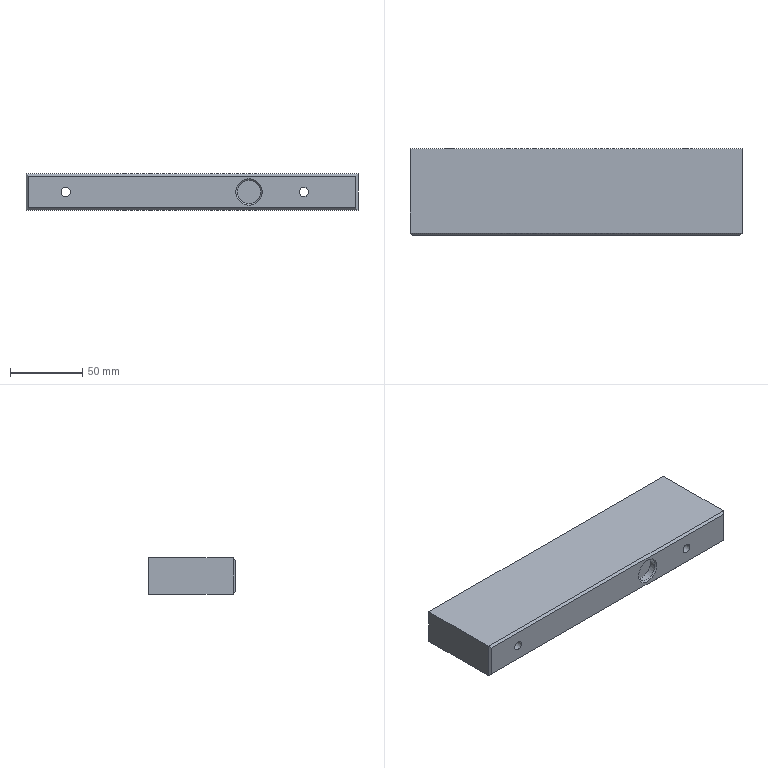Part | NX | 1 solid | 15 faces | box 230 x 60 x 25 mm | volume 339289 mm3 | plane 11 | cylinder 3 | cone 1 | commonest cylinder face diameters 6.5 x2 16.2 x1
STEP:
#1=CARTESIAN_POINT('',(0.,1.5,25.));
#2=VERTEX_POINT('',#1);
#3=CARTESIAN_POINT('',(0.,60.,25.));
#4=VERTEX_POINT('',#3);
#5=CARTESIAN_POINT('',(0.,30.,25.));
#6=DIRECTION('',(0.,1.,0.));
#7=VECTOR('',#6,1000.);
#8=LINE('',#5,#7);
#9=EDGE_CURVE('',#2,#4,#8,.T.);
#10=ORIENTED_EDGE('',*,*,#9,.F.);
#11=CARTESIAN_POINT('',(230.,1.5,25.));
#12=VERTEX_POINT('',#11);
#13=CARTESIAN_POINT('',(115.,1.5,25.));
#14=DIRECTION('',(1.,0.,0.));
#15=VECTOR('',#14,1000.);
#16=LINE('',#13,#15);
#17=EDGE_CURVE('',#2,#12,#16,.T.);
#18=ORIENTED_EDGE('',*,*,#17,.T.);
#19=CARTESIAN_POINT('',(230.,60.,25.));
#20=VERTEX_POINT('',#19);
#21=CARTESIAN_POINT('',(230.,30.,25.));
#22=DIRECTION('',(0.,-1.,0.));
#23=VECTOR('',#22,1000.);
#24=LINE('',#21,#23);
#25=EDGE_CURVE('',#20,#12,#24,.T.);
#26=ORIENTED_EDGE('',*,*,#25,.F.);
#27=CARTESIAN_POINT('',(115.,60.,25.));
#28=DIRECTION('',(1.,0.,0.));
#29=VECTOR('',#28,1000.);
#30=LINE('',#27,#29);
#31=EDGE_CURVE('',#4,#20,#30,.T.);
#32=ORIENTED_EDGE('',*,*,#31,.F.);
#33=EDGE_LOOP('',(#10,#18,#26,#32));
#34=FACE_BOUND('',#33,.T.);
#35=CARTESIAN_POINT('',(115.,30.,25.));
#36=DIRECTION('',(0.,0.,1.));
#37=DIRECTION('',(1.,0.,0.));
#38=AXIS2_PLACEMENT_3D('',#35,#36,#37);
#39=PLANE('',#38);
#40=ADVANCED_FACE('',(#34),#39,.T.);
#41=CARTESIAN_POINT('',(228.5,0.,1.5));
#42=VERTEX_POINT('',#41);
#43=CARTESIAN_POINT('',(228.5,0.,23.5));
#44=VERTEX_POINT('',#43);
#45=CARTESIAN_POINT('',(228.5,0.,0.));
#46=DIRECTION('',(0.,0.,1.));
#47=VECTOR('',#46,1000.);
#48=LINE('',#45,#47);
#49=EDGE_CURVE('',#42,#44,#48,.T.);
#50=ORIENTED_EDGE('',*,*,#49,.T.);
#51=CARTESIAN_POINT('',(1.5,0.,23.5));
#52=VERTEX_POINT('',#51);
#53=CARTESIAN_POINT('',(115.,0.,23.5));
#54=DIRECTION('',(-1.,0.,0.));
#55=VECTOR('',#54,1000.);
#56=LINE('',#53,#55);
#57=EDGE_CURVE('',#44,#52,#56,.T.);
#58=ORIENTED_EDGE('',*,*,#57,.T.);
#59=CARTESIAN_POINT('',(1.5,0.,1.5));
#60=VERTEX_POINT('',#59);
#61=CARTESIAN_POINT('',(1.5,0.,0.));
#62=DIRECTION('',(0.,0.,-1.));
#63=VECTOR('',#62,1000.);
#64=LINE('',#61,#63);
#65=EDGE_CURVE('',#52,#60,#64,.T.);
#66=ORIENTED_EDGE('',*,*,#65,.T.);
#67=CARTESIAN_POINT('',(115.,0.,1.5));
#68=DIRECTION('',(1.,0.,0.));
#69=VECTOR('',#68,1000.);
#70=LINE('',#67,#69);
#71=EDGE_CURVE('',#60,#42,#70,.T.);
#72=ORIENTED_EDGE('',*,*,#71,.T.);
#73=EDGE_LOOP('',(#50,#58,#66,#72));
#74=FACE_BOUND('',#73,.T.);
#75=CARTESIAN_POINT('',(154.5,0.,3.4));
#76=VERTEX_POINT('',#75);
#77=CARTESIAN_POINT('',(154.5,0.,12.5));
#78=DIRECTION('',(0.,-1.,0.));
#79=DIRECTION('',(0.,0.,-1.));
#80=AXIS2_PLACEMENT_3D('',#77,#78,#79);
#81=CIRCLE('',#80,9.1);
#82=EDGE_CURVE('',#76,#76,#81,.F.);
#83=ORIENTED_EDGE('',*,*,#82,.T.);
#84=EDGE_LOOP('',(#83));
#85=FACE_BOUND('',#84,.T.);
#86=CARTESIAN_POINT('',(192.5,0.,15.75));
#87=VERTEX_POINT('',#86);
#88=CARTESIAN_POINT('',(192.5,0.,12.5));
#89=DIRECTION('',(0.,1.,0.));
#90=DIRECTION('',(0.,0.,1.));
#91=AXIS2_PLACEMENT_3D('',#88,#89,#90);
#92=CIRCLE('',#91,3.25);
#93=EDGE_CURVE('',#87,#87,#92,.T.);
#94=ORIENTED_EDGE('',*,*,#93,.T.);
#95=EDGE_LOOP('',(#94));
#96=FACE_BOUND('',#95,.T.);
#97=CARTESIAN_POINT('',(27.5,0.,15.75));
#98=VERTEX_POINT('',#97);
#99=CARTESIAN_POINT('',(27.5,0.,12.5));
#100=DIRECTION('',(0.,1.,0.));
#101=DIRECTION('',(0.,0.,1.));
#102=AXIS2_PLACEMENT_3D('',#99,#100,#101);
#103=CIRCLE('',#102,3.25);
#104=EDGE_CURVE('',#98,#98,#103,.T.);
#105=ORIENTED_EDGE('',*,*,#104,.T.);
#106=EDGE_LOOP('',(#105));
#107=FACE_BOUND('',#106,.T.);
#108=CARTESIAN_POINT('',(115.,0.,0.));
#109=DIRECTION('',(0.,-1.,0.));
#110=DIRECTION('',(0.,0.,-1.));
#111=AXIS2_PLACEMENT_3D('',#108,#109,#110);
#112=PLANE('',#111);
#113=ADVANCED_FACE('',(#74,#85,#96,#107),#112,.T.);
#114=CARTESIAN_POINT('',(0.,60.,0.));
#115=VERTEX_POINT('',#114);
#116=CARTESIAN_POINT('',(0.,1.5,0.));
#117=VERTEX_POINT('',#116);
#118=CARTESIAN_POINT('',(0.,30.,0.));
#119=DIRECTION('',(0.,-1.,0.));
#120=VECTOR('',#119,1000.);
#121=LINE('',#118,#120);
#122=EDGE_CURVE('',#115,#117,#121,.T.);
#123=ORIENTED_EDGE('',*,*,#122,.T.);
#124=CARTESIAN_POINT('',(0.,1.5,0.));
#125=DIRECTION('',(0.,0.,1.));
#126=VECTOR('',#125,1000.);
#127=LINE('',#124,#126);
#128=EDGE_CURVE('',#117,#2,#127,.T.);
#129=ORIENTED_EDGE('',*,*,#128,.T.);
#130=ORIENTED_EDGE('',*,*,#9,.T.);
#131=CARTESIAN_POINT('',(0.,60.,0.));
#132=DIRECTION('',(0.,0.,1.));
#133=VECTOR('',#132,1000.);
#134=LINE('',#131,#133);
#135=EDGE_CURVE('',#115,#4,#134,.T.);
#136=ORIENTED_EDGE('',*,*,#135,.F.);
#137=EDGE_LOOP('',(#123,#129,#130,#136));
#138=FACE_BOUND('',#137,.T.);
#139=CARTESIAN_POINT('',(0.,30.,0.));
#140=DIRECTION('',(-1.,0.,0.));
#141=DIRECTION('',(0.,0.,1.));
#142=AXIS2_PLACEMENT_3D('',#139,#140,#141);
#143=PLANE('',#142);
#144=ADVANCED_FACE('',(#138),#143,.T.);
#145=CARTESIAN_POINT('',(192.5,60.,15.75));
#146=VERTEX_POINT('',#145);
#147=CARTESIAN_POINT('',(192.5,60.,12.5));
#148=DIRECTION('',(0.,1.,0.));
#149=DIRECTION('',(0.,0.,1.));
#150=AXIS2_PLACEMENT_3D('',#147,#148,#149);
#151=CIRCLE('',#150,3.25);
#152=EDGE_CURVE('',#146,#146,#151,.T.);
#153=ORIENTED_EDGE('',*,*,#152,.F.);
#154=EDGE_LOOP('',(#153));
#155=FACE_BOUND('',#154,.T.);
#156=CARTESIAN_POINT('',(27.5,60.,15.75));
#157=VERTEX_POINT('',#156);
#158=CARTESIAN_POINT('',(27.5,60.,12.5));
#159=DIRECTION('',(0.,1.,0.));
#160=DIRECTION('',(0.,0.,1.));
#161=AXIS2_PLACEMENT_3D('',#158,#159,#160);
#162=CIRCLE('',#161,3.25);
#163=EDGE_CURVE('',#157,#157,#162,.T.);
#164=ORIENTED_EDGE('',*,*,#163,.F.);
#165=EDGE_LOOP('',(#164));
#166=FACE_BOUND('',#165,.T.);
#167=ORIENTED_EDGE('',*,*,#135,.T.);
#168=ORIENTED_EDGE('',*,*,#31,.T.);
#169=CARTESIAN_POINT('',(230.,60.,0.));
#170=VERTEX_POINT('',#169);
#171=CARTESIAN_POINT('',(230.,60.,0.));
#172=DIRECTION('',(0.,0.,1.));
#173=VECTOR('',#172,1000.);
#174=LINE('',#171,#173);
#175=EDGE_CURVE('',#170,#20,#174,.T.);
#176=ORIENTED_EDGE('',*,*,#175,.F.);
#177=CARTESIAN_POINT('',(115.,60.,0.));
#178=DIRECTION('',(-1.,0.,0.));
#179=VECTOR('',#178,1000.);
#180=LINE('',#177,#179);
#181=EDGE_CURVE('',#170,#115,#180,.T.);
#182=ORIENTED_EDGE('',*,*,#181,.T.);
#183=EDGE_LOOP('',(#167,#168,#176,#182));
#184=FACE_BOUND('',#183,.T.);
#185=CARTESIAN_POINT('',(115.,60.,0.));
#186=DIRECTION('',(0.,1.,0.));
#187=DIRECTION('',(0.,0.,1.));
#188=AXIS2_PLACEMENT_3D('',#185,#186,#187);
#189=PLANE('',#188);
#190=ADVANCED_FACE('',(#155,#166,#184),#189,.T.);
#191=CARTESIAN_POINT('',(230.,1.5,0.));
#192=VERTEX_POINT('',#191);
#193=CARTESIAN_POINT('',(230.,30.,0.));
#194=DIRECTION('',(0.,1.,0.));
#195=VECTOR('',#194,1000.);
#196=LINE('',#193,#195);
#197=EDGE_CURVE('',#192,#170,#196,.T.);
#198=ORIENTED_EDGE('',*,*,#197,.F.);
#199=CARTESIAN_POINT('',(115.,1.5,0.));
#200=DIRECTION('',(-1.,0.,0.));
#201=VECTOR('',#200,1000.);
#202=LINE('',#199,#201);
#203=EDGE_CURVE('',#192,#117,#202,.T.);
#204=ORIENTED_EDGE('',*,*,#203,.T.);
#205=ORIENTED_EDGE('',*,*,#122,.F.);
#206=ORIENTED_EDGE('',*,*,#181,.F.);
#207=EDGE_LOOP('',(#198,#204,#205,#206));
#208=FACE_BOUND('',#207,.T.);
#209=CARTESIAN_POINT('',(115.,30.,0.));
#210=DIRECTION('',(0.,0.,-1.));
#211=DIRECTION('',(-1.,0.,0.));
#212=AXIS2_PLACEMENT_3D('',#209,#210,#211);
#213=PLANE('',#212);
#214=ADVANCED_FACE('',(#208),#213,.T.);
#215=ORIENTED_EDGE('',*,*,#25,.T.);
#216=CARTESIAN_POINT('',(230.,1.5,0.));
#217=DIRECTION('',(0.,0.,-1.));
#218=VECTOR('',#217,1000.);
#219=LINE('',#216,#218);
#220=EDGE_CURVE('',#12,#192,#219,.T.);
#221=ORIENTED_EDGE('',*,*,#220,.T.);
#222=ORIENTED_EDGE('',*,*,#197,.T.);
#223=ORIENTED_EDGE('',*,*,#175,.T.);
#224=EDGE_LOOP('',(#215,#221,#222,#223));
#225=FACE_BOUND('',#224,.T.);
#226=CARTESIAN_POINT('',(230.,30.,0.));
#227=DIRECTION('',(1.,0.,0.));
#228=DIRECTION('',(0.,0.,-1.));
#229=AXIS2_PLACEMENT_3D('',#226,#227,#228);
#230=PLANE('',#229);
#231=ADVANCED_FACE('',(#225),#230,.T.);
#232=ORIENTED_EDGE('',*,*,#163,.T.);
#233=EDGE_LOOP('',(#232));
#234=FACE_BOUND('',#233,.T.);
#235=ORIENTED_EDGE('',*,*,#104,.F.);
#236=EDGE_LOOP('',(#235));
#237=FACE_BOUND('',#236,.T.);
#238=CARTESIAN_POINT('',(27.5,0.,12.5));
#239=DIRECTION('',(0.,1.,0.));
#240=DIRECTION('',(0.,0.,1.));
#241=AXIS2_PLACEMENT_3D('',#238,#239,#240);
#242=CYLINDRICAL_SURFACE('',#241,3.25);
#243=ADVANCED_FACE('',(#234,#237),#242,.F.);
#244=ORIENTED_EDGE('',*,*,#152,.T.);
#245=EDGE_LOOP('',(#244));
#246=FACE_BOUND('',#245,.T.);
#247=ORIENTED_EDGE('',*,*,#93,.F.);
#248=EDGE_LOOP('',(#247));
#249=FACE_BOUND('',#248,.T.);
#250=CARTESIAN_POINT('',(192.5,0.,12.5));
#251=DIRECTION('',(0.,1.,0.));
#252=DIRECTION('',(0.,0.,1.));
#253=AXIS2_PLACEMENT_3D('',#250,#251,#252);
#254=CYLINDRICAL_SURFACE('',#253,3.25);
#255=ADVANCED_FACE('',(#246,#249),#254,.F.);
#256=CARTESIAN_POINT('',(154.5,5.5,20.6));
#257=VERTEX_POINT('',#256);
#258=CARTESIAN_POINT('',(154.5,5.5,12.5));
#259=DIRECTION('',(0.,1.,0.));
#260=DIRECTION('',(0.,0.,1.));
#261=AXIS2_PLACEMENT_3D('',#258,#259,#260);
#262=CIRCLE('',#261,8.1);
#263=EDGE_CURVE('',#257,#257,#262,.F.);
#264=ORIENTED_EDGE('',*,*,#263,.T.);
#265=EDGE_LOOP('',(#264));
#266=FACE_BOUND('',#265,.T.);
#267=CARTESIAN_POINT('',(154.5,5.5,12.5));
#268=DIRECTION('',(0.,1.,0.));
#269=DIRECTION('',(0.,0.,1.));
#270=AXIS2_PLACEMENT_3D('',#267,#268,#269);
#271=PLANE('',#270);
#272=ADVANCED_FACE('',(#266),#271,.F.);
#273=CARTESIAN_POINT('',(154.5,1.,4.4));
#274=VERTEX_POINT('',#273);
#275=CARTESIAN_POINT('',(154.5,1.,12.5));
#276=DIRECTION('',(0.,-1.,0.));
#277=DIRECTION('',(0.,0.,-1.));
#278=AXIS2_PLACEMENT_3D('',#275,#276,#277);
#279=CIRCLE('',#278,8.1);
#280=EDGE_CURVE('',#274,#274,#279,.T.);
#281=ORIENTED_EDGE('',*,*,#280,.T.);
#282=EDGE_LOOP('',(#281));
#283=FACE_BOUND('',#282,.T.);
#284=ORIENTED_EDGE('',*,*,#263,.F.);
#285=EDGE_LOOP('',(#284));
#286=FACE_BOUND('',#285,.T.);
#287=CARTESIAN_POINT('',(154.5,0.,12.5));
#288=DIRECTION('',(0.,1.,0.));
#289=DIRECTION('',(0.,0.,1.));
#290=AXIS2_PLACEMENT_3D('',#287,#288,#289);
#291=CYLINDRICAL_SURFACE('',#290,8.1);
#292=ADVANCED_FACE('',(#283,#286),#291,.F.);
#293=ORIENTED_EDGE('',*,*,#280,.F.);
#294=EDGE_LOOP('',(#293));
#295=FACE_BOUND('',#294,.T.);
#296=ORIENTED_EDGE('',*,*,#82,.F.);
#297=EDGE_LOOP('',(#296));
#298=FACE_BOUND('',#297,.T.);
#299=CARTESIAN_POINT('',(154.5,0.,12.5));
#300=DIRECTION('',(0.,-1.,0.));
#301=DIRECTION('',(0.,0.,-1.));
#302=AXIS2_PLACEMENT_3D('',#299,#300,#301);
#303=CONICAL_SURFACE('',#302,9.1,0.7854);
#304=ADVANCED_FACE('',(#295,#298),#303,.F.);
#305=CARTESIAN_POINT('',(39.333,-37.833,39.333));
#306=DIRECTION('',(-0.5774,0.5774,-0.5774));
#307=VECTOR('',#306,1000.);
#308=LINE('',#305,#307);
#309=EDGE_CURVE('',#117,#60,#308,.F.);
#310=ORIENTED_EDGE('',*,*,#309,.F.);
#311=ORIENTED_EDGE('',*,*,#203,.F.);
#312=CARTESIAN_POINT('',(229.,0.5,1.));
#313=DIRECTION('',(0.5774,0.5774,-0.5774));
#314=VECTOR('',#313,1000.);
#315=LINE('',#312,#314);
#316=EDGE_CURVE('',#42,#192,#315,.T.);
#317=ORIENTED_EDGE('',*,*,#316,.F.);
#318=ORIENTED_EDGE('',*,*,#71,.F.);
#319=EDGE_LOOP('',(#310,#311,#317,#318));
#320=FACE_BOUND('',#319,.T.);
#321=CARTESIAN_POINT('',(115.,0.,1.5));
#322=DIRECTION('',(0.,0.7071,0.7071));
#323=DIRECTION('',(1.,0.,0.));
#324=AXIS2_PLACEMENT_3D('',#321,#322,#323);
#325=PLANE('',#324);
#326=ADVANCED_FACE('',(#320),#325,.F.);
#327=ORIENTED_EDGE('',*,*,#316,.T.);
#328=ORIENTED_EDGE('',*,*,#220,.F.);
#329=CARTESIAN_POINT('',(220.667,-7.833,15.667));
#330=DIRECTION('',(-0.5774,-0.5774,-0.5774));
#331=VECTOR('',#330,1000.);
#332=LINE('',#329,#331);
#333=EDGE_CURVE('',#44,#12,#332,.F.);
#334=ORIENTED_EDGE('',*,*,#333,.F.);
#335=ORIENTED_EDGE('',*,*,#49,.F.);
#336=EDGE_LOOP('',(#327,#328,#334,#335));
#337=FACE_BOUND('',#336,.T.);
#338=CARTESIAN_POINT('',(228.5,0.,0.));
#339=DIRECTION('',(-0.7071,0.7071,0.));
#340=DIRECTION('',(0.,0.,1.));
#341=AXIS2_PLACEMENT_3D('',#338,#339,#340);
#342=PLANE('',#341);
#343=ADVANCED_FACE('',(#337),#342,.F.);
#344=ORIENTED_EDGE('',*,*,#309,.T.);
#345=ORIENTED_EDGE('',*,*,#65,.F.);
#346=CARTESIAN_POINT('',(8.333,-6.833,16.667));
#347=DIRECTION('',(-0.5774,0.5774,0.5774));
#348=VECTOR('',#347,1000.);
#349=LINE('',#346,#348);
#350=EDGE_CURVE('',#2,#52,#349,.F.);
#351=ORIENTED_EDGE('',*,*,#350,.F.);
#352=ORIENTED_EDGE('',*,*,#128,.F.);
#353=EDGE_LOOP('',(#344,#345,#351,#352));
#354=FACE_BOUND('',#353,.T.);
#355=CARTESIAN_POINT('',(0.,1.5,0.));
#356=DIRECTION('',(0.7071,0.7071,0.));
#357=DIRECTION('',(0.,0.,1.));
#358=AXIS2_PLACEMENT_3D('',#355,#356,#357);
#359=PLANE('',#358);
#360=ADVANCED_FACE('',(#354),#359,.F.);
#361=ORIENTED_EDGE('',*,*,#333,.T.);
#362=ORIENTED_EDGE('',*,*,#17,.F.);
#363=ORIENTED_EDGE('',*,*,#350,.T.);
#364=ORIENTED_EDGE('',*,*,#57,.F.);
#365=EDGE_LOOP('',(#361,#362,#363,#364));
#366=FACE_BOUND('',#365,.T.);
#367=CARTESIAN_POINT('',(115.,0.,23.5));
#368=DIRECTION('',(0.,0.7071,-0.7071));
#369=DIRECTION('',(-1.,0.,0.));
#370=AXIS2_PLACEMENT_3D('',#367,#368,#369);
#371=PLANE('',#370);
#372=ADVANCED_FACE('',(#366),#371,.F.);
#373=CLOSED_SHELL('',(#40,#113,#144,#190,#214,#231,#243,#255,#272,#292,#304,#326,#343,#360,#372));
#374=MANIFOLD_SOLID_BREP('',#373);
#375=(LENGTH_UNIT()NAMED_UNIT(*)SI_UNIT(.MILLI.,.METRE.));
#376=UNCERTAINTY_MEASURE_WITH_UNIT(LENGTH_MEASURE(0.00001),#375,'','');
#377=(NAMED_UNIT(*)PLANE_ANGLE_UNIT()SI_UNIT($,.RADIAN.));
#378=(NAMED_UNIT(*)SI_UNIT($,.STERADIAN.)SOLID_ANGLE_UNIT());
#379=(GEOMETRIC_REPRESENTATION_CONTEXT(3)GLOBAL_UNCERTAINTY_ASSIGNED_CONTEXT((#376))GLOBAL_UNIT_ASSIGNED_CONTEXT((#375,#377,#378))REPRESENTATION_CONTEXT('',''));
#380=ADVANCED_BREP_SHAPE_REPRESENTATION('',(#374),#379);